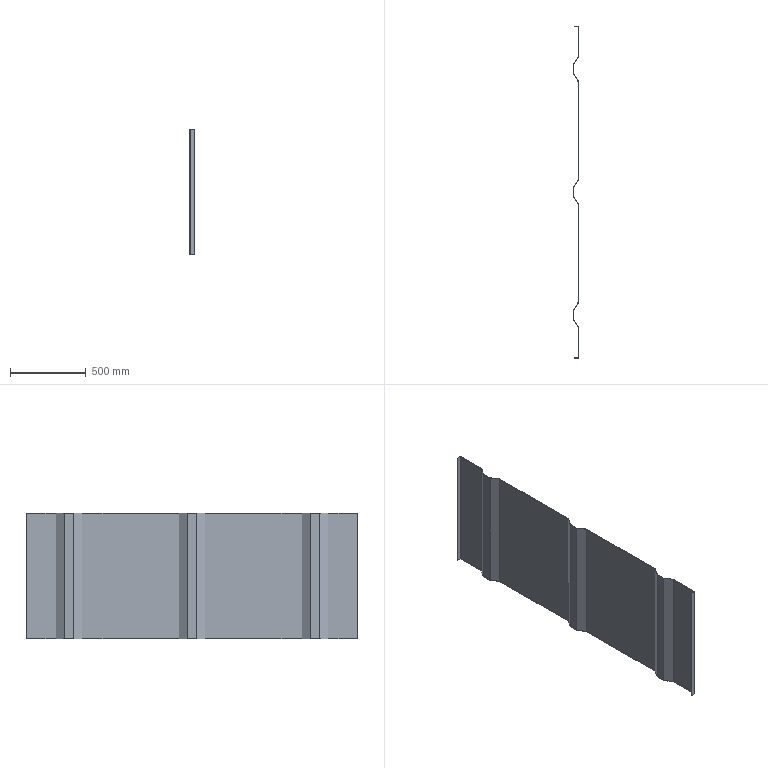Part | SolidWorks | features ExtruThin 1, ICE 1 | 1 solid | 34 faces | box 38 x 2190 x 827 mm | volume 3823055 mm3 | plane 34
STEP:
#1=CARTESIAN_POINT('',(-2.,-1093.,-413.5));
#2=VERTEX_POINT('',#1);
#3=CARTESIAN_POINT('',(-30.,-1093.,-413.5));
#4=VERTEX_POINT('',#3);
#5=CARTESIAN_POINT('',(0.,-1093.,-413.5));
#6=DIRECTION('',(-1.,0.,0.));
#7=VECTOR('',#6,1000.);
#8=LINE('',#5,#7);
#9=EDGE_CURVE('',#2,#4,#8,.T.);
#10=ORIENTED_EDGE('',*,*,#9,.T.);
#11=CARTESIAN_POINT('',(-30.,-1093.,413.5));
#12=VERTEX_POINT('',#11);
#13=CARTESIAN_POINT('',(-30.,-1093.,413.5));
#14=DIRECTION('',(0.,0.,-1.));
#15=VECTOR('',#14,1000.);
#16=LINE('',#13,#15);
#17=EDGE_CURVE('',#12,#4,#16,.T.);
#18=ORIENTED_EDGE('',*,*,#17,.F.);
#19=CARTESIAN_POINT('',(-2.,-1093.,413.5));
#20=VERTEX_POINT('',#19);
#21=CARTESIAN_POINT('',(0.,-1093.,413.5));
#22=DIRECTION('',(-1.,0.,0.));
#23=VECTOR('',#22,1000.);
#24=LINE('',#21,#23);
#25=EDGE_CURVE('',#20,#12,#24,.T.);
#26=ORIENTED_EDGE('',*,*,#25,.F.);
#27=CARTESIAN_POINT('',(-2.,-1093.,413.5));
#28=DIRECTION('',(0.,0.,-1.));
#29=VECTOR('',#28,1000.);
#30=LINE('',#27,#29);
#31=EDGE_CURVE('',#20,#2,#30,.T.);
#32=ORIENTED_EDGE('',*,*,#31,.T.);
#33=EDGE_LOOP('',(#10,#18,#26,#32));
#34=FACE_OUTER_BOUND('',#33,.T.);
#35=CARTESIAN_POINT('',(0.,-1093.,413.5));
#36=DIRECTION('',(0.,-1.,0.));
#37=DIRECTION('',(0.,0.,-1.));
#38=AXIS2_PLACEMENT_3D('',#35,#36,#37);
#39=PLANE('',#38);
#40=ADVANCED_FACE('',(#34),#39,.F.);
#41=CARTESIAN_POINT('',(-30.,-1095.,-413.5));
#42=VERTEX_POINT('',#41);
#43=CARTESIAN_POINT('',(-30.,-1095.,-413.5));
#44=DIRECTION('',(0.,1.,0.));
#45=VECTOR('',#44,1000.);
#46=LINE('',#43,#45);
#47=EDGE_CURVE('',#42,#4,#46,.T.);
#48=ORIENTED_EDGE('',*,*,#47,.F.);
#49=CARTESIAN_POINT('',(-30.,-1095.,413.5));
#50=VERTEX_POINT('',#49);
#51=CARTESIAN_POINT('',(-30.,-1095.,413.5));
#52=DIRECTION('',(0.,0.,-1.));
#53=VECTOR('',#52,1000.);
#54=LINE('',#51,#53);
#55=EDGE_CURVE('',#50,#42,#54,.T.);
#56=ORIENTED_EDGE('',*,*,#55,.F.);
#57=CARTESIAN_POINT('',(-30.,-1095.,413.5));
#58=DIRECTION('',(0.,1.,0.));
#59=VECTOR('',#58,1000.);
#60=LINE('',#57,#59);
#61=EDGE_CURVE('',#50,#12,#60,.T.);
#62=ORIENTED_EDGE('',*,*,#61,.T.);
#63=ORIENTED_EDGE('',*,*,#17,.T.);
#64=EDGE_LOOP('',(#48,#56,#62,#63));
#65=FACE_OUTER_BOUND('',#64,.T.);
#66=CARTESIAN_POINT('',(-30.,-1095.,413.5));
#67=DIRECTION('',(-1.,0.,0.));
#68=DIRECTION('',(0.,0.,1.));
#69=AXIS2_PLACEMENT_3D('',#66,#67,#68);
#70=PLANE('',#69);
#71=ADVANCED_FACE('',(#65),#70,.T.);
#72=CARTESIAN_POINT('',(0.,-1095.,-413.5));
#73=VERTEX_POINT('',#72);
#74=CARTESIAN_POINT('',(0.,-1095.,-413.5));
#75=DIRECTION('',(-1.,0.,0.));
#76=VECTOR('',#75,1000.);
#77=LINE('',#74,#76);
#78=EDGE_CURVE('',#73,#42,#77,.T.);
#79=ORIENTED_EDGE('',*,*,#78,.F.);
#80=CARTESIAN_POINT('',(0.,-1095.,413.5));
#81=VERTEX_POINT('',#80);
#82=CARTESIAN_POINT('',(0.,-1095.,413.5));
#83=DIRECTION('',(0.,0.,-1.));
#84=VECTOR('',#83,1000.);
#85=LINE('',#82,#84);
#86=EDGE_CURVE('',#81,#73,#85,.T.);
#87=ORIENTED_EDGE('',*,*,#86,.F.);
#88=CARTESIAN_POINT('',(0.,-1095.,413.5));
#89=DIRECTION('',(-1.,0.,0.));
#90=VECTOR('',#89,1000.);
#91=LINE('',#88,#90);
#92=EDGE_CURVE('',#81,#50,#91,.T.);
#93=ORIENTED_EDGE('',*,*,#92,.T.);
#94=ORIENTED_EDGE('',*,*,#55,.T.);
#95=EDGE_LOOP('',(#79,#87,#93,#94));
#96=FACE_OUTER_BOUND('',#95,.T.);
#97=CARTESIAN_POINT('',(0.,-1095.,413.5));
#98=DIRECTION('',(0.,-1.,0.));
#99=DIRECTION('',(0.,0.,-1.));
#100=AXIS2_PLACEMENT_3D('',#97,#98,#99);
#101=PLANE('',#100);
#102=ADVANCED_FACE('',(#96),#101,.T.);
#103=CARTESIAN_POINT('',(0.,-895.,-413.5));
#104=VERTEX_POINT('',#103);
#105=CARTESIAN_POINT('',(0.,-895.,-413.5));
#106=DIRECTION('',(0.,-1.,0.));
#107=VECTOR('',#106,1000.);
#108=LINE('',#105,#107);
#109=EDGE_CURVE('',#104,#73,#108,.T.);
#110=ORIENTED_EDGE('',*,*,#109,.F.);
#111=CARTESIAN_POINT('',(0.,-895.,413.5));
#112=VERTEX_POINT('',#111);
#113=CARTESIAN_POINT('',(0.,-895.,413.5));
#114=DIRECTION('',(0.,0.,-1.));
#115=VECTOR('',#114,1000.);
#116=LINE('',#113,#115);
#117=EDGE_CURVE('',#112,#104,#116,.T.);
#118=ORIENTED_EDGE('',*,*,#117,.F.);
#119=CARTESIAN_POINT('',(0.,-895.,413.5));
#120=DIRECTION('',(0.,-1.,0.));
#121=VECTOR('',#120,1000.);
#122=LINE('',#119,#121);
#123=EDGE_CURVE('',#112,#81,#122,.T.);
#124=ORIENTED_EDGE('',*,*,#123,.T.);
#125=ORIENTED_EDGE('',*,*,#86,.T.);
#126=EDGE_LOOP('',(#110,#118,#124,#125));
#127=FACE_OUTER_BOUND('',#126,.T.);
#128=CARTESIAN_POINT('',(0.,-895.,413.5));
#129=DIRECTION('',(1.,0.,0.));
#130=DIRECTION('',(0.,1.,0.));
#131=AXIS2_PLACEMENT_3D('',#128,#129,#130);
#132=PLANE('',#131);
#133=ADVANCED_FACE('',(#127),#132,.T.);
#134=CARTESIAN_POINT('',(-36.,-841.,-413.5));
#135=VERTEX_POINT('',#134);
#136=CARTESIAN_POINT('',(0.,-895.,-413.5));
#137=DIRECTION('',(0.5547,-0.8321,0.));
#138=VECTOR('',#137,1000.);
#139=LINE('',#136,#138);
#140=EDGE_CURVE('',#135,#104,#139,.T.);
#141=ORIENTED_EDGE('',*,*,#140,.F.);
#142=CARTESIAN_POINT('',(-36.,-841.,413.5));
#143=VERTEX_POINT('',#142);
#144=CARTESIAN_POINT('',(-36.,-841.,413.5));
#145=DIRECTION('',(0.,0.,-1.));
#146=VECTOR('',#145,1000.);
#147=LINE('',#144,#146);
#148=EDGE_CURVE('',#143,#135,#147,.T.);
#149=ORIENTED_EDGE('',*,*,#148,.F.);
#150=CARTESIAN_POINT('',(0.,-895.,413.5));
#151=DIRECTION('',(0.5547,-0.8321,0.));
#152=VECTOR('',#151,1000.);
#153=LINE('',#150,#152);
#154=EDGE_CURVE('',#143,#112,#153,.T.);
#155=ORIENTED_EDGE('',*,*,#154,.T.);
#156=ORIENTED_EDGE('',*,*,#117,.T.);
#157=EDGE_LOOP('',(#141,#149,#155,#156));
#158=FACE_OUTER_BOUND('',#157,.T.);
#159=CARTESIAN_POINT('',(0.,-895.,413.5));
#160=DIRECTION('',(0.8321,0.5547,0.));
#161=DIRECTION('',(-0.5547,0.8321,0.));
#162=AXIS2_PLACEMENT_3D('',#159,#160,#161);
#163=PLANE('',#162);
#164=ADVANCED_FACE('',(#158),#163,.T.);
#165=CARTESIAN_POINT('',(-36.,-781.,-413.5));
#166=VERTEX_POINT('',#165);
#167=CARTESIAN_POINT('',(-36.,-841.,-413.5));
#168=DIRECTION('',(0.,-1.,0.));
#169=VECTOR('',#168,1000.);
#170=LINE('',#167,#169);
#171=EDGE_CURVE('',#166,#135,#170,.T.);
#172=ORIENTED_EDGE('',*,*,#171,.F.);
#173=CARTESIAN_POINT('',(-36.,-781.,413.5));
#174=VERTEX_POINT('',#173);
#175=CARTESIAN_POINT('',(-36.,-781.,413.5));
#176=DIRECTION('',(0.,0.,-1.));
#177=VECTOR('',#176,1000.);
#178=LINE('',#175,#177);
#179=EDGE_CURVE('',#174,#166,#178,.T.);
#180=ORIENTED_EDGE('',*,*,#179,.F.);
#181=CARTESIAN_POINT('',(-36.,-841.,413.5));
#182=DIRECTION('',(0.,-1.,0.));
#183=VECTOR('',#182,1000.);
#184=LINE('',#181,#183);
#185=EDGE_CURVE('',#174,#143,#184,.T.);
#186=ORIENTED_EDGE('',*,*,#185,.T.);
#187=ORIENTED_EDGE('',*,*,#148,.T.);
#188=EDGE_LOOP('',(#172,#180,#186,#187));
#189=FACE_OUTER_BOUND('',#188,.T.);
#190=CARTESIAN_POINT('',(-36.,-841.,413.5));
#191=DIRECTION('',(1.,0.,0.));
#192=DIRECTION('',(0.,1.,0.));
#193=AXIS2_PLACEMENT_3D('',#190,#191,#192);
#194=PLANE('',#193);
#195=ADVANCED_FACE('',(#189),#194,.T.);
#196=CARTESIAN_POINT('',(0.,-727.,-413.5));
#197=VERTEX_POINT('',#196);
#198=CARTESIAN_POINT('',(-36.,-781.,-413.5));
#199=DIRECTION('',(-0.5547,-0.8321,0.));
#200=VECTOR('',#199,1000.);
#201=LINE('',#198,#200);
#202=EDGE_CURVE('',#197,#166,#201,.T.);
#203=ORIENTED_EDGE('',*,*,#202,.F.);
#204=CARTESIAN_POINT('',(0.,-727.,413.5));
#205=VERTEX_POINT('',#204);
#206=CARTESIAN_POINT('',(0.,-727.,413.5));
#207=DIRECTION('',(0.,0.,-1.));
#208=VECTOR('',#207,1000.);
#209=LINE('',#206,#208);
#210=EDGE_CURVE('',#205,#197,#209,.T.);
#211=ORIENTED_EDGE('',*,*,#210,.F.);
#212=CARTESIAN_POINT('',(-36.,-781.,413.5));
#213=DIRECTION('',(-0.5547,-0.8321,0.));
#214=VECTOR('',#213,1000.);
#215=LINE('',#212,#214);
#216=EDGE_CURVE('',#205,#174,#215,.T.);
#217=ORIENTED_EDGE('',*,*,#216,.T.);
#218=ORIENTED_EDGE('',*,*,#179,.T.);
#219=EDGE_LOOP('',(#203,#211,#217,#218));
#220=FACE_OUTER_BOUND('',#219,.T.);
#221=CARTESIAN_POINT('',(-36.,-781.,413.5));
#222=DIRECTION('',(0.8321,-0.5547,0.));
#223=DIRECTION('',(0.5547,0.8321,0.));
#224=AXIS2_PLACEMENT_3D('',#221,#222,#223);
#225=PLANE('',#224);
#226=ADVANCED_FACE('',(#220),#225,.T.);
#227=CARTESIAN_POINT('',(0.,-84.,-413.5));
#228=VERTEX_POINT('',#227);
#229=CARTESIAN_POINT('',(0.,-84.,-413.5));
#230=DIRECTION('',(0.,-1.,0.));
#231=VECTOR('',#230,1000.);
#232=LINE('',#229,#231);
#233=EDGE_CURVE('',#228,#197,#232,.T.);
#234=ORIENTED_EDGE('',*,*,#233,.F.);
#235=CARTESIAN_POINT('',(0.,-84.,413.5));
#236=VERTEX_POINT('',#235);
#237=CARTESIAN_POINT('',(0.,-84.,413.5));
#238=DIRECTION('',(0.,0.,-1.));
#239=VECTOR('',#238,1000.);
#240=LINE('',#237,#239);
#241=EDGE_CURVE('',#236,#228,#240,.T.);
#242=ORIENTED_EDGE('',*,*,#241,.F.);
#243=CARTESIAN_POINT('',(0.,-84.,413.5));
#244=DIRECTION('',(0.,-1.,0.));
#245=VECTOR('',#244,1000.);
#246=LINE('',#243,#245);
#247=EDGE_CURVE('',#236,#205,#246,.T.);
#248=ORIENTED_EDGE('',*,*,#247,.T.);
#249=ORIENTED_EDGE('',*,*,#210,.T.);
#250=EDGE_LOOP('',(#234,#242,#248,#249));
#251=FACE_OUTER_BOUND('',#250,.T.);
#252=CARTESIAN_POINT('',(0.,-84.,413.5));
#253=DIRECTION('',(1.,0.,0.));
#254=DIRECTION('',(0.,1.,0.));
#255=AXIS2_PLACEMENT_3D('',#252,#253,#254);
#256=PLANE('',#255);
#257=ADVANCED_FACE('',(#251),#256,.T.);
#258=CARTESIAN_POINT('',(-36.,-30.,-413.5));
#259=VERTEX_POINT('',#258);
#260=CARTESIAN_POINT('',(-36.,-30.,-413.5));
#261=DIRECTION('',(0.5547,-0.8321,0.));
#262=VECTOR('',#261,1000.);
#263=LINE('',#260,#262);
#264=EDGE_CURVE('',#259,#228,#263,.T.);
#265=ORIENTED_EDGE('',*,*,#264,.F.);
#266=CARTESIAN_POINT('',(-36.,-30.,413.5));
#267=VERTEX_POINT('',#266);
#268=CARTESIAN_POINT('',(-36.,-30.,413.5));
#269=DIRECTION('',(0.,0.,-1.));
#270=VECTOR('',#269,1000.);
#271=LINE('',#268,#270);
#272=EDGE_CURVE('',#267,#259,#271,.T.);
#273=ORIENTED_EDGE('',*,*,#272,.F.);
#274=CARTESIAN_POINT('',(-36.,-30.,413.5));
#275=DIRECTION('',(0.5547,-0.8321,0.));
#276=VECTOR('',#275,1000.);
#277=LINE('',#274,#276);
#278=EDGE_CURVE('',#267,#236,#277,.T.);
#279=ORIENTED_EDGE('',*,*,#278,.T.);
#280=ORIENTED_EDGE('',*,*,#241,.T.);
#281=EDGE_LOOP('',(#265,#273,#279,#280));
#282=FACE_OUTER_BOUND('',#281,.T.);
#283=CARTESIAN_POINT('',(-36.,-30.,413.5));
#284=DIRECTION('',(0.8321,0.5547,0.));
#285=DIRECTION('',(-0.5547,0.8321,0.));
#286=AXIS2_PLACEMENT_3D('',#283,#284,#285);
#287=PLANE('',#286);
#288=ADVANCED_FACE('',(#282),#287,.T.);
#289=CARTESIAN_POINT('',(-36.,30.,-413.5));
#290=VERTEX_POINT('',#289);
#291=CARTESIAN_POINT('',(-36.,30.,-413.5));
#292=DIRECTION('',(0.,-1.,0.));
#293=VECTOR('',#292,1000.);
#294=LINE('',#291,#293);
#295=EDGE_CURVE('',#290,#259,#294,.T.);
#296=ORIENTED_EDGE('',*,*,#295,.F.);
#297=CARTESIAN_POINT('',(-36.,30.,413.5));
#298=VERTEX_POINT('',#297);
#299=CARTESIAN_POINT('',(-36.,30.,413.5));
#300=DIRECTION('',(0.,0.,-1.));
#301=VECTOR('',#300,1000.);
#302=LINE('',#299,#301);
#303=EDGE_CURVE('',#298,#290,#302,.T.);
#304=ORIENTED_EDGE('',*,*,#303,.F.);
#305=CARTESIAN_POINT('',(-36.,30.,413.5));
#306=DIRECTION('',(0.,-1.,0.));
#307=VECTOR('',#306,1000.);
#308=LINE('',#305,#307);
#309=EDGE_CURVE('',#298,#267,#308,.T.);
#310=ORIENTED_EDGE('',*,*,#309,.T.);
#311=ORIENTED_EDGE('',*,*,#272,.T.);
#312=EDGE_LOOP('',(#296,#304,#310,#311));
#313=FACE_OUTER_BOUND('',#312,.T.);
#314=CARTESIAN_POINT('',(-36.,30.,413.5));
#315=DIRECTION('',(1.,0.,0.));
#316=DIRECTION('',(0.,1.,0.));
#317=AXIS2_PLACEMENT_3D('',#314,#315,#316);
#318=PLANE('',#317);
#319=ADVANCED_FACE('',(#313),#318,.T.);
#320=CARTESIAN_POINT('',(0.,84.,-413.5));
#321=VERTEX_POINT('',#320);
#322=CARTESIAN_POINT('',(0.,84.,-413.5));
#323=DIRECTION('',(-0.5547,-0.8321,0.));
#324=VECTOR('',#323,1000.);
#325=LINE('',#322,#324);
#326=EDGE_CURVE('',#321,#290,#325,.T.);
#327=ORIENTED_EDGE('',*,*,#326,.F.);
#328=CARTESIAN_POINT('',(0.,84.,413.5));
#329=VERTEX_POINT('',#328);
#330=CARTESIAN_POINT('',(0.,84.,413.5));
#331=DIRECTION('',(0.,0.,-1.));
#332=VECTOR('',#331,1000.);
#333=LINE('',#330,#332);
#334=EDGE_CURVE('',#329,#321,#333,.T.);
#335=ORIENTED_EDGE('',*,*,#334,.F.);
#336=CARTESIAN_POINT('',(0.,84.,413.5));
#337=DIRECTION('',(-0.5547,-0.8321,0.));
#338=VECTOR('',#337,1000.);
#339=LINE('',#336,#338);
#340=EDGE_CURVE('',#329,#298,#339,.T.);
#341=ORIENTED_EDGE('',*,*,#340,.T.);
#342=ORIENTED_EDGE('',*,*,#303,.T.);
#343=EDGE_LOOP('',(#327,#335,#341,#342));
#344=FACE_OUTER_BOUND('',#343,.T.);
#345=CARTESIAN_POINT('',(0.,84.,413.5));
#346=DIRECTION('',(0.8321,-0.5547,0.));
#347=DIRECTION('',(0.5547,0.8321,0.));
#348=AXIS2_PLACEMENT_3D('',#345,#346,#347);
#349=PLANE('',#348);
#350=ADVANCED_FACE('',(#344),#349,.T.);
#351=CARTESIAN_POINT('',(0.,727.,-413.5));
#352=VERTEX_POINT('',#351);
#353=CARTESIAN_POINT('',(0.,727.,-413.5));
#354=DIRECTION('',(0.,-1.,0.));
#355=VECTOR('',#354,1000.);
#356=LINE('',#353,#355);
#357=EDGE_CURVE('',#352,#321,#356,.T.);
#358=ORIENTED_EDGE('',*,*,#357,.F.);
#359=CARTESIAN_POINT('',(0.,727.,413.5));
#360=VERTEX_POINT('',#359);
#361=CARTESIAN_POINT('',(0.,727.,413.5));
#362=DIRECTION('',(0.,0.,-1.));
#363=VECTOR('',#362,1000.);
#364=LINE('',#361,#363);
#365=EDGE_CURVE('',#360,#352,#364,.T.);
#366=ORIENTED_EDGE('',*,*,#365,.F.);
#367=CARTESIAN_POINT('',(0.,727.,413.5));
#368=DIRECTION('',(0.,-1.,0.));
#369=VECTOR('',#368,1000.);
#370=LINE('',#367,#369);
#371=EDGE_CURVE('',#360,#329,#370,.T.);
#372=ORIENTED_EDGE('',*,*,#371,.T.);
#373=ORIENTED_EDGE('',*,*,#334,.T.);
#374=EDGE_LOOP('',(#358,#366,#372,#373));
#375=FACE_OUTER_BOUND('',#374,.T.);
#376=CARTESIAN_POINT('',(0.,727.,413.5));
#377=DIRECTION('',(1.,0.,0.));
#378=DIRECTION('',(0.,1.,0.));
#379=AXIS2_PLACEMENT_3D('',#376,#377,#378);
#380=PLANE('',#379);
#381=ADVANCED_FACE('',(#375),#380,.T.);
#382=CARTESIAN_POINT('',(-36.,781.,-413.5));
#383=VERTEX_POINT('',#382);
#384=CARTESIAN_POINT('',(-36.,781.,-413.5));
#385=DIRECTION('',(0.5547,-0.8321,0.));
#386=VECTOR('',#385,1000.);
#387=LINE('',#384,#386);
#388=EDGE_CURVE('',#383,#352,#387,.T.);
#389=ORIENTED_EDGE('',*,*,#388,.F.);
#390=CARTESIAN_POINT('',(-36.,781.,413.5));
#391=VERTEX_POINT('',#390);
#392=CARTESIAN_POINT('',(-36.,781.,413.5));
#393=DIRECTION('',(0.,0.,-1.));
#394=VECTOR('',#393,1000.);
#395=LINE('',#392,#394);
#396=EDGE_CURVE('',#391,#383,#395,.T.);
#397=ORIENTED_EDGE('',*,*,#396,.F.);
#398=CARTESIAN_POINT('',(-36.,781.,413.5));
#399=DIRECTION('',(0.5547,-0.8321,0.));
#400=VECTOR('',#399,1000.);
#401=LINE('',#398,#400);
#402=EDGE_CURVE('',#391,#360,#401,.T.);
#403=ORIENTED_EDGE('',*,*,#402,.T.);
#404=ORIENTED_EDGE('',*,*,#365,.T.);
#405=EDGE_LOOP('',(#389,#397,#403,#404));
#406=FACE_OUTER_BOUND('',#405,.T.);
#407=CARTESIAN_POINT('',(-36.,781.,413.5));
#408=DIRECTION('',(0.8321,0.5547,0.));
#409=DIRECTION('',(-0.5547,0.8321,0.));
#410=AXIS2_PLACEMENT_3D('',#407,#408,#409);
#411=PLANE('',#410);
#412=ADVANCED_FACE('',(#406),#411,.T.);
#413=CARTESIAN_POINT('',(-36.,841.,-413.5));
#414=VERTEX_POINT('',#413);
#415=CARTESIAN_POINT('',(-36.,841.,-413.5));
#416=DIRECTION('',(0.,-1.,0.));
#417=VECTOR('',#416,1000.);
#418=LINE('',#415,#417);
#419=EDGE_CURVE('',#414,#383,#418,.T.);
#420=ORIENTED_EDGE('',*,*,#419,.F.);
#421=CARTESIAN_POINT('',(-36.,841.,413.5));
#422=VERTEX_POINT('',#421);
#423=CARTESIAN_POINT('',(-36.,841.,413.5));
#424=DIRECTION('',(0.,0.,-1.));
#425=VECTOR('',#424,1000.);
#426=LINE('',#423,#425);
#427=EDGE_CURVE('',#422,#414,#426,.T.);
#428=ORIENTED_EDGE('',*,*,#427,.F.);
#429=CARTESIAN_POINT('',(-36.,841.,413.5));
#430=DIRECTION('',(0.,-1.,0.));
#431=VECTOR('',#430,1000.);
#432=LINE('',#429,#431);
#433=EDGE_CURVE('',#422,#391,#432,.T.);
#434=ORIENTED_EDGE('',*,*,#433,.T.);
#435=ORIENTED_EDGE('',*,*,#396,.T.);
#436=EDGE_LOOP('',(#420,#428,#434,#435));
#437=FACE_OUTER_BOUND('',#436,.T.);
#438=CARTESIAN_POINT('',(-36.,841.,413.5));
#439=DIRECTION('',(1.,0.,0.));
#440=DIRECTION('',(0.,1.,0.));
#441=AXIS2_PLACEMENT_3D('',#438,#439,#440);
#442=PLANE('',#441);
#443=ADVANCED_FACE('',(#437),#442,.T.);
#444=CARTESIAN_POINT('',(0.,895.,-413.5));
#445=VERTEX_POINT('',#444);
#446=CARTESIAN_POINT('',(0.,895.,-413.5));
#447=DIRECTION('',(-0.5547,-0.8321,0.));
#448=VECTOR('',#447,1000.);
#449=LINE('',#446,#448);
#450=EDGE_CURVE('',#445,#414,#449,.T.);
#451=ORIENTED_EDGE('',*,*,#450,.F.);
#452=CARTESIAN_POINT('',(0.,895.,413.5));
#453=VERTEX_POINT('',#452);
#454=CARTESIAN_POINT('',(0.,895.,413.5));
#455=DIRECTION('',(0.,0.,-1.));
#456=VECTOR('',#455,1000.);
#457=LINE('',#454,#456);
#458=EDGE_CURVE('',#453,#445,#457,.T.);
#459=ORIENTED_EDGE('',*,*,#458,.F.);
#460=CARTESIAN_POINT('',(0.,895.,413.5));
#461=DIRECTION('',(-0.5547,-0.8321,0.));
#462=VECTOR('',#461,1000.);
#463=LINE('',#460,#462);
#464=EDGE_CURVE('',#453,#422,#463,.T.);
#465=ORIENTED_EDGE('',*,*,#464,.T.);
#466=ORIENTED_EDGE('',*,*,#427,.T.);
#467=EDGE_LOOP('',(#451,#459,#465,#466));
#468=FACE_OUTER_BOUND('',#467,.T.);
#469=CARTESIAN_POINT('',(0.,895.,413.5));
#470=DIRECTION('',(0.8321,-0.5547,0.));
#471=DIRECTION('',(0.5547,0.8321,0.));
#472=AXIS2_PLACEMENT_3D('',#469,#470,#471);
#473=PLANE('',#472);
#474=ADVANCED_FACE('',(#468),#473,.T.);
#475=CARTESIAN_POINT('',(0.,1095.,-413.5));
#476=VERTEX_POINT('',#475);
#477=CARTESIAN_POINT('',(0.,1095.,-413.5));
#478=DIRECTION('',(0.,-1.,0.));
#479=VECTOR('',#478,1000.);
#480=LINE('',#477,#479);
#481=EDGE_CURVE('',#476,#445,#480,.T.);
#482=ORIENTED_EDGE('',*,*,#481,.F.);
#483=CARTESIAN_POINT('',(0.,1095.,413.5));
#484=VERTEX_POINT('',#483);
#485=CARTESIAN_POINT('',(0.,1095.,413.5));
#486=DIRECTION('',(0.,0.,-1.));
#487=VECTOR('',#486,1000.);
#488=LINE('',#485,#487);
#489=EDGE_CURVE('',#484,#476,#488,.T.);
#490=ORIENTED_EDGE('',*,*,#489,.F.);
#491=CARTESIAN_POINT('',(0.,1095.,413.5));
#492=DIRECTION('',(0.,-1.,0.));
#493=VECTOR('',#492,1000.);
#494=LINE('',#491,#493);
#495=EDGE_CURVE('',#484,#453,#494,.T.);
#496=ORIENTED_EDGE('',*,*,#495,.T.);
#497=ORIENTED_EDGE('',*,*,#458,.T.);
#498=EDGE_LOOP('',(#482,#490,#496,#497));
#499=FACE_OUTER_BOUND('',#498,.T.);
#500=CARTESIAN_POINT('',(0.,1095.,413.5));
#501=DIRECTION('',(1.,0.,0.));
#502=DIRECTION('',(0.,1.,0.));
#503=AXIS2_PLACEMENT_3D('',#500,#501,#502);
#504=PLANE('',#503);
#505=ADVANCED_FACE('',(#499),#504,.T.);
#506=CARTESIAN_POINT('',(-30.,1095.,-413.5));
#507=VERTEX_POINT('',#506);
#508=CARTESIAN_POINT('',(0.,1095.,-413.5));
#509=DIRECTION('',(1.,0.,0.));
#510=VECTOR('',#509,1000.);
#511=LINE('',#508,#510);
#512=EDGE_CURVE('',#507,#476,#511,.T.);
#513=ORIENTED_EDGE('',*,*,#512,.F.);
#514=CARTESIAN_POINT('',(-30.,1095.,413.5));
#515=VERTEX_POINT('',#514);
#516=CARTESIAN_POINT('',(-30.,1095.,413.5));
#517=DIRECTION('',(0.,0.,-1.));
#518=VECTOR('',#517,1000.);
#519=LINE('',#516,#518);
#520=EDGE_CURVE('',#515,#507,#519,.T.);
#521=ORIENTED_EDGE('',*,*,#520,.F.);
#522=CARTESIAN_POINT('',(0.,1095.,413.5));
#523=DIRECTION('',(1.,0.,0.));
#524=VECTOR('',#523,1000.);
#525=LINE('',#522,#524);
#526=EDGE_CURVE('',#515,#484,#525,.T.);
#527=ORIENTED_EDGE('',*,*,#526,.T.);
#528=ORIENTED_EDGE('',*,*,#489,.T.);
#529=EDGE_LOOP('',(#513,#521,#527,#528));
#530=FACE_OUTER_BOUND('',#529,.T.);
#531=CARTESIAN_POINT('',(0.,1095.,413.5));
#532=DIRECTION('',(0.,1.,0.));
#533=DIRECTION('',(0.,0.,1.));
#534=AXIS2_PLACEMENT_3D('',#531,#532,#533);
#535=PLANE('',#534);
#536=ADVANCED_FACE('',(#530),#535,.T.);
#537=CARTESIAN_POINT('',(-30.,1093.,-413.5));
#538=VERTEX_POINT('',#537);
#539=CARTESIAN_POINT('',(-30.,1093.,-413.5));
#540=DIRECTION('',(0.,1.,0.));
#541=VECTOR('',#540,1000.);
#542=LINE('',#539,#541);
#543=EDGE_CURVE('',#538,#507,#542,.T.);
#544=ORIENTED_EDGE('',*,*,#543,.F.);
#545=CARTESIAN_POINT('',(-30.,1093.,413.5));
#546=VERTEX_POINT('',#545);
#547=CARTESIAN_POINT('',(-30.,1093.,413.5));
#548=DIRECTION('',(0.,0.,-1.));
#549=VECTOR('',#548,1000.);
#550=LINE('',#547,#549);
#551=EDGE_CURVE('',#546,#538,#550,.T.);
#552=ORIENTED_EDGE('',*,*,#551,.F.);
#553=CARTESIAN_POINT('',(-30.,1093.,413.5));
#554=DIRECTION('',(0.,1.,0.));
#555=VECTOR('',#554,1000.);
#556=LINE('',#553,#555);
#557=EDGE_CURVE('',#546,#515,#556,.T.);
#558=ORIENTED_EDGE('',*,*,#557,.T.);
#559=ORIENTED_EDGE('',*,*,#520,.T.);
#560=EDGE_LOOP('',(#544,#552,#558,#559));
#561=FACE_OUTER_BOUND('',#560,.T.);
#562=CARTESIAN_POINT('',(-30.,1093.,413.5));
#563=DIRECTION('',(-1.,0.,0.));
#564=DIRECTION('',(0.,0.,1.));
#565=AXIS2_PLACEMENT_3D('',#562,#563,#564);
#566=PLANE('',#565);
#567=ADVANCED_FACE('',(#561),#566,.T.);
#568=CARTESIAN_POINT('',(-2.,1093.,-413.5));
#569=VERTEX_POINT('',#568);
#570=CARTESIAN_POINT('',(0.,1093.,-413.5));
#571=DIRECTION('',(1.,0.,0.));
#572=VECTOR('',#571,1000.);
#573=LINE('',#570,#572);
#574=EDGE_CURVE('',#538,#569,#573,.T.);
#575=ORIENTED_EDGE('',*,*,#574,.T.);
#576=CARTESIAN_POINT('',(-2.,1093.,413.5));
#577=VERTEX_POINT('',#576);
#578=CARTESIAN_POINT('',(-2.,1093.,413.5));
#579=DIRECTION('',(0.,0.,-1.));
#580=VECTOR('',#579,1000.);
#581=LINE('',#578,#580);
#582=EDGE_CURVE('',#577,#569,#581,.T.);
#583=ORIENTED_EDGE('',*,*,#582,.F.);
#584=CARTESIAN_POINT('',(0.,1093.,413.5));
#585=DIRECTION('',(1.,0.,0.));
#586=VECTOR('',#585,1000.);
#587=LINE('',#584,#586);
#588=EDGE_CURVE('',#546,#577,#587,.T.);
#589=ORIENTED_EDGE('',*,*,#588,.F.);
#590=ORIENTED_EDGE('',*,*,#551,.T.);
#591=EDGE_LOOP('',(#575,#583,#589,#590));
#592=FACE_OUTER_BOUND('',#591,.T.);
#593=CARTESIAN_POINT('',(0.,1093.,413.5));
#594=DIRECTION('',(0.,1.,0.));
#595=DIRECTION('',(0.,0.,1.));
#596=AXIS2_PLACEMENT_3D('',#593,#594,#595);
#597=PLANE('',#596);
#598=ADVANCED_FACE('',(#592),#597,.F.);
#599=CARTESIAN_POINT('',(-2.,895.606,-413.5));
#600=VERTEX_POINT('',#599);
#601=CARTESIAN_POINT('',(-2.,1095.,-413.5));
#602=DIRECTION('',(0.,-1.,0.));
#603=VECTOR('',#602,1000.);
#604=LINE('',#601,#603);
#605=EDGE_CURVE('',#569,#600,#604,.T.);
#606=ORIENTED_EDGE('',*,*,#605,.T.);
#607=CARTESIAN_POINT('',(-2.,895.606,413.5));
#608=VERTEX_POINT('',#607);
#609=CARTESIAN_POINT('',(-2.,895.606,413.5));
#610=DIRECTION('',(0.,0.,-1.));
#611=VECTOR('',#610,1000.);
#612=LINE('',#609,#611);
#613=EDGE_CURVE('',#608,#600,#612,.T.);
#614=ORIENTED_EDGE('',*,*,#613,.F.);
#615=CARTESIAN_POINT('',(-2.,1095.,413.5));
#616=DIRECTION('',(0.,-1.,0.));
#617=VECTOR('',#616,1000.);
#618=LINE('',#615,#617);
#619=EDGE_CURVE('',#577,#608,#618,.T.);
#620=ORIENTED_EDGE('',*,*,#619,.F.);
#621=ORIENTED_EDGE('',*,*,#582,.T.);
#622=EDGE_LOOP('',(#606,#614,#620,#621));
#623=FACE_OUTER_BOUND('',#622,.T.);
#624=CARTESIAN_POINT('',(-2.,1095.,413.5));
#625=DIRECTION('',(1.,0.,0.));
#626=DIRECTION('',(0.,1.,0.));
#627=AXIS2_PLACEMENT_3D('',#624,#625,#626);
#628=PLANE('',#627);
#629=ADVANCED_FACE('',(#623),#628,.F.);
#630=CARTESIAN_POINT('',(-38.,841.606,-413.5));
#631=VERTEX_POINT('',#630);
#632=CARTESIAN_POINT('',(-1.664,896.109,-413.5));
#633=DIRECTION('',(-0.5547,-0.8321,0.));
#634=VECTOR('',#633,1000.);
#635=LINE('',#632,#634);
#636=EDGE_CURVE('',#600,#631,#635,.T.);
#637=ORIENTED_EDGE('',*,*,#636,.T.);
#638=CARTESIAN_POINT('',(-38.,841.606,413.5));
#639=VERTEX_POINT('',#638);
#640=CARTESIAN_POINT('',(-38.,841.606,413.5));
#641=DIRECTION('',(0.,0.,-1.));
#642=VECTOR('',#641,1000.);
#643=LINE('',#640,#642);
#644=EDGE_CURVE('',#639,#631,#643,.T.);
#645=ORIENTED_EDGE('',*,*,#644,.F.);
#646=CARTESIAN_POINT('',(-1.664,896.109,413.5));
#647=DIRECTION('',(-0.5547,-0.8321,0.));
#648=VECTOR('',#647,1000.);
#649=LINE('',#646,#648);
#650=EDGE_CURVE('',#608,#639,#649,.T.);
#651=ORIENTED_EDGE('',*,*,#650,.F.);
#652=ORIENTED_EDGE('',*,*,#613,.T.);
#653=EDGE_LOOP('',(#637,#645,#651,#652));
#654=FACE_OUTER_BOUND('',#653,.T.);
#655=CARTESIAN_POINT('',(-1.664,896.109,413.5));
#656=DIRECTION('',(0.8321,-0.5547,0.));
#657=DIRECTION('',(0.5547,0.8321,0.));
#658=AXIS2_PLACEMENT_3D('',#655,#656,#657);
#659=PLANE('',#658);
#660=ADVANCED_FACE('',(#654),#659,.F.);
#661=CARTESIAN_POINT('',(-38.,780.394,-413.5));
#662=VERTEX_POINT('',#661);
#663=CARTESIAN_POINT('',(-38.,841.,-413.5));
#664=DIRECTION('',(0.,-1.,0.));
#665=VECTOR('',#664,1000.);
#666=LINE('',#663,#665);
#667=EDGE_CURVE('',#631,#662,#666,.T.);
#668=ORIENTED_EDGE('',*,*,#667,.T.);
#669=CARTESIAN_POINT('',(-38.,780.394,413.5));
#670=VERTEX_POINT('',#669);
#671=CARTESIAN_POINT('',(-38.,780.394,413.5));
#672=DIRECTION('',(0.,0.,-1.));
#673=VECTOR('',#672,1000.);
#674=LINE('',#671,#673);
#675=EDGE_CURVE('',#670,#662,#674,.T.);
#676=ORIENTED_EDGE('',*,*,#675,.F.);
#677=CARTESIAN_POINT('',(-38.,841.,413.5));
#678=DIRECTION('',(0.,-1.,0.));
#679=VECTOR('',#678,1000.);
#680=LINE('',#677,#679);
#681=EDGE_CURVE('',#639,#670,#680,.T.);
#682=ORIENTED_EDGE('',*,*,#681,.F.);
#683=ORIENTED_EDGE('',*,*,#644,.T.);
#684=EDGE_LOOP('',(#668,#676,#682,#683));
#685=FACE_OUTER_BOUND('',#684,.T.);
#686=CARTESIAN_POINT('',(-38.,841.,413.5));
#687=DIRECTION('',(1.,0.,0.));
#688=DIRECTION('',(0.,1.,0.));
#689=AXIS2_PLACEMENT_3D('',#686,#687,#688);
#690=PLANE('',#689);
#691=ADVANCED_FACE('',(#685),#690,.F.);
#692=CARTESIAN_POINT('',(-2.,726.394,-413.5));
#693=VERTEX_POINT('',#692);
#694=CARTESIAN_POINT('',(-37.664,779.891,-413.5));
#695=DIRECTION('',(0.5547,-0.8321,0.));
#696=VECTOR('',#695,1000.);
#697=LINE('',#694,#696);
#698=EDGE_CURVE('',#662,#693,#697,.T.);
#699=ORIENTED_EDGE('',*,*,#698,.T.);
#700=CARTESIAN_POINT('',(-2.,726.394,413.5));
#701=VERTEX_POINT('',#700);
#702=CARTESIAN_POINT('',(-2.,726.394,413.5));
#703=DIRECTION('',(0.,0.,-1.));
#704=VECTOR('',#703,1000.);
#705=LINE('',#702,#704);
#706=EDGE_CURVE('',#701,#693,#705,.T.);
#707=ORIENTED_EDGE('',*,*,#706,.F.);
#708=CARTESIAN_POINT('',(-37.664,779.891,413.5));
#709=DIRECTION('',(0.5547,-0.8321,0.));
#710=VECTOR('',#709,1000.);
#711=LINE('',#708,#710);
#712=EDGE_CURVE('',#670,#701,#711,.T.);
#713=ORIENTED_EDGE('',*,*,#712,.F.);
#714=ORIENTED_EDGE('',*,*,#675,.T.);
#715=EDGE_LOOP('',(#699,#707,#713,#714));
#716=FACE_OUTER_BOUND('',#715,.T.);
#717=CARTESIAN_POINT('',(-37.664,779.891,413.5));
#718=DIRECTION('',(0.8321,0.5547,0.));
#719=DIRECTION('',(-0.5547,0.8321,0.));
#720=AXIS2_PLACEMENT_3D('',#717,#718,#719);
#721=PLANE('',#720);
#722=ADVANCED_FACE('',(#716),#721,.F.);
#723=CARTESIAN_POINT('',(-2.,84.606,-413.5));
#724=VERTEX_POINT('',#723);
#725=CARTESIAN_POINT('',(-2.,727.,-413.5));
#726=DIRECTION('',(0.,-1.,0.));
#727=VECTOR('',#726,1000.);
#728=LINE('',#725,#727);
#729=EDGE_CURVE('',#693,#724,#728,.T.);
#730=ORIENTED_EDGE('',*,*,#729,.T.);
#731=CARTESIAN_POINT('',(-2.,84.606,413.5));
#732=VERTEX_POINT('',#731);
#733=CARTESIAN_POINT('',(-2.,84.606,413.5));
#734=DIRECTION('',(0.,0.,-1.));
#735=VECTOR('',#734,1000.);
#736=LINE('',#733,#735);
#737=EDGE_CURVE('',#732,#724,#736,.T.);
#738=ORIENTED_EDGE('',*,*,#737,.F.);
#739=CARTESIAN_POINT('',(-2.,727.,413.5));
#740=DIRECTION('',(0.,-1.,0.));
#741=VECTOR('',#740,1000.);
#742=LINE('',#739,#741);
#743=EDGE_CURVE('',#701,#732,#742,.T.);
#744=ORIENTED_EDGE('',*,*,#743,.F.);
#745=ORIENTED_EDGE('',*,*,#706,.T.);
#746=EDGE_LOOP('',(#730,#738,#744,#745));
#747=FACE_OUTER_BOUND('',#746,.T.);
#748=CARTESIAN_POINT('',(-2.,727.,413.5));
#749=DIRECTION('',(1.,0.,0.));
#750=DIRECTION('',(0.,1.,0.));
#751=AXIS2_PLACEMENT_3D('',#748,#749,#750);
#752=PLANE('',#751);
#753=ADVANCED_FACE('',(#747),#752,.F.);
#754=CARTESIAN_POINT('',(-38.,30.606,-413.5));
#755=VERTEX_POINT('',#754);
#756=CARTESIAN_POINT('',(-1.664,85.109,-413.5));
#757=DIRECTION('',(-0.5547,-0.8321,0.));
#758=VECTOR('',#757,1000.);
#759=LINE('',#756,#758);
#760=EDGE_CURVE('',#724,#755,#759,.T.);
#761=ORIENTED_EDGE('',*,*,#760,.T.);
#762=CARTESIAN_POINT('',(-38.,30.606,413.5));
#763=VERTEX_POINT('',#762);
#764=CARTESIAN_POINT('',(-38.,30.606,413.5));
#765=DIRECTION('',(0.,0.,-1.));
#766=VECTOR('',#765,1000.);
#767=LINE('',#764,#766);
#768=EDGE_CURVE('',#763,#755,#767,.T.);
#769=ORIENTED_EDGE('',*,*,#768,.F.);
#770=CARTESIAN_POINT('',(-1.664,85.109,413.5));
#771=DIRECTION('',(-0.5547,-0.8321,0.));
#772=VECTOR('',#771,1000.);
#773=LINE('',#770,#772);
#774=EDGE_CURVE('',#732,#763,#773,.T.);
#775=ORIENTED_EDGE('',*,*,#774,.F.);
#776=ORIENTED_EDGE('',*,*,#737,.T.);
#777=EDGE_LOOP('',(#761,#769,#775,#776));
#778=FACE_OUTER_BOUND('',#777,.T.);
#779=CARTESIAN_POINT('',(-1.664,85.109,413.5));
#780=DIRECTION('',(0.8321,-0.5547,0.));
#781=DIRECTION('',(0.5547,0.8321,0.));
#782=AXIS2_PLACEMENT_3D('',#779,#780,#781);
#783=PLANE('',#782);
#784=ADVANCED_FACE('',(#778),#783,.F.);
#785=CARTESIAN_POINT('',(-38.,-30.606,-413.5));
#786=VERTEX_POINT('',#785);
#787=CARTESIAN_POINT('',(-38.,30.,-413.5));
#788=DIRECTION('',(0.,-1.,0.));
#789=VECTOR('',#788,1000.);
#790=LINE('',#787,#789);
#791=EDGE_CURVE('',#755,#786,#790,.T.);
#792=ORIENTED_EDGE('',*,*,#791,.T.);
#793=CARTESIAN_POINT('',(-38.,-30.606,413.5));
#794=VERTEX_POINT('',#793);
#795=CARTESIAN_POINT('',(-38.,-30.606,413.5));
#796=DIRECTION('',(0.,0.,-1.));
#797=VECTOR('',#796,1000.);
#798=LINE('',#795,#797);
#799=EDGE_CURVE('',#794,#786,#798,.T.);
#800=ORIENTED_EDGE('',*,*,#799,.F.);
#801=CARTESIAN_POINT('',(-38.,30.,413.5));
#802=DIRECTION('',(0.,-1.,0.));
#803=VECTOR('',#802,1000.);
#804=LINE('',#801,#803);
#805=EDGE_CURVE('',#763,#794,#804,.T.);
#806=ORIENTED_EDGE('',*,*,#805,.F.);
#807=ORIENTED_EDGE('',*,*,#768,.T.);
#808=EDGE_LOOP('',(#792,#800,#806,#807));
#809=FACE_OUTER_BOUND('',#808,.T.);
#810=CARTESIAN_POINT('',(-38.,30.,413.5));
#811=DIRECTION('',(1.,0.,0.));
#812=DIRECTION('',(0.,1.,0.));
#813=AXIS2_PLACEMENT_3D('',#810,#811,#812);
#814=PLANE('',#813);
#815=ADVANCED_FACE('',(#809),#814,.F.);
#816=CARTESIAN_POINT('',(-2.,-84.606,-413.5));
#817=VERTEX_POINT('',#816);
#818=CARTESIAN_POINT('',(-37.664,-31.109,-413.5));
#819=DIRECTION('',(0.5547,-0.8321,0.));
#820=VECTOR('',#819,1000.);
#821=LINE('',#818,#820);
#822=EDGE_CURVE('',#786,#817,#821,.T.);
#823=ORIENTED_EDGE('',*,*,#822,.T.);
#824=CARTESIAN_POINT('',(-2.,-84.606,413.5));
#825=VERTEX_POINT('',#824);
#826=CARTESIAN_POINT('',(-2.,-84.606,413.5));
#827=DIRECTION('',(0.,0.,-1.));
#828=VECTOR('',#827,1000.);
#829=LINE('',#826,#828);
#830=EDGE_CURVE('',#825,#817,#829,.T.);
#831=ORIENTED_EDGE('',*,*,#830,.F.);
#832=CARTESIAN_POINT('',(-37.664,-31.109,413.5));
#833=DIRECTION('',(0.5547,-0.8321,0.));
#834=VECTOR('',#833,1000.);
#835=LINE('',#832,#834);
#836=EDGE_CURVE('',#794,#825,#835,.T.);
#837=ORIENTED_EDGE('',*,*,#836,.F.);
#838=ORIENTED_EDGE('',*,*,#799,.T.);
#839=EDGE_LOOP('',(#823,#831,#837,#838));
#840=FACE_OUTER_BOUND('',#839,.T.);
#841=CARTESIAN_POINT('',(-37.664,-31.109,413.5));
#842=DIRECTION('',(0.8321,0.5547,0.));
#843=DIRECTION('',(-0.5547,0.8321,0.));
#844=AXIS2_PLACEMENT_3D('',#841,#842,#843);
#845=PLANE('',#844);
#846=ADVANCED_FACE('',(#840),#845,.F.);
#847=CARTESIAN_POINT('',(-2.,-726.394,-413.5));
#848=VERTEX_POINT('',#847);
#849=CARTESIAN_POINT('',(-2.,-84.,-413.5));
#850=DIRECTION('',(0.,-1.,0.));
#851=VECTOR('',#850,1000.);
#852=LINE('',#849,#851);
#853=EDGE_CURVE('',#817,#848,#852,.T.);
#854=ORIENTED_EDGE('',*,*,#853,.T.);
#855=CARTESIAN_POINT('',(-2.,-726.394,413.5));
#856=VERTEX_POINT('',#855);
#857=CARTESIAN_POINT('',(-2.,-726.394,413.5));
#858=DIRECTION('',(0.,0.,-1.));
#859=VECTOR('',#858,1000.);
#860=LINE('',#857,#859);
#861=EDGE_CURVE('',#856,#848,#860,.T.);
#862=ORIENTED_EDGE('',*,*,#861,.F.);
#863=CARTESIAN_POINT('',(-2.,-84.,413.5));
#864=DIRECTION('',(0.,-1.,0.));
#865=VECTOR('',#864,1000.);
#866=LINE('',#863,#865);
#867=EDGE_CURVE('',#825,#856,#866,.T.);
#868=ORIENTED_EDGE('',*,*,#867,.F.);
#869=ORIENTED_EDGE('',*,*,#830,.T.);
#870=EDGE_LOOP('',(#854,#862,#868,#869));
#871=FACE_OUTER_BOUND('',#870,.T.);
#872=CARTESIAN_POINT('',(-2.,-84.,413.5));
#873=DIRECTION('',(1.,0.,0.));
#874=DIRECTION('',(0.,1.,0.));
#875=AXIS2_PLACEMENT_3D('',#872,#873,#874);
#876=PLANE('',#875);
#877=ADVANCED_FACE('',(#871),#876,.F.);
#878=CARTESIAN_POINT('',(-38.,-780.394,-413.5));
#879=VERTEX_POINT('',#878);
#880=CARTESIAN_POINT('',(-37.664,-779.891,-413.5));
#881=DIRECTION('',(-0.5547,-0.8321,0.));
#882=VECTOR('',#881,1000.);
#883=LINE('',#880,#882);
#884=EDGE_CURVE('',#848,#879,#883,.T.);
#885=ORIENTED_EDGE('',*,*,#884,.T.);
#886=CARTESIAN_POINT('',(-38.,-780.394,413.5));
#887=VERTEX_POINT('',#886);
#888=CARTESIAN_POINT('',(-38.,-780.394,413.5));
#889=DIRECTION('',(0.,0.,-1.));
#890=VECTOR('',#889,1000.);
#891=LINE('',#888,#890);
#892=EDGE_CURVE('',#887,#879,#891,.T.);
#893=ORIENTED_EDGE('',*,*,#892,.F.);
#894=CARTESIAN_POINT('',(-37.664,-779.891,413.5));
#895=DIRECTION('',(-0.5547,-0.8321,0.));
#896=VECTOR('',#895,1000.);
#897=LINE('',#894,#896);
#898=EDGE_CURVE('',#856,#887,#897,.T.);
#899=ORIENTED_EDGE('',*,*,#898,.F.);
#900=ORIENTED_EDGE('',*,*,#861,.T.);
#901=EDGE_LOOP('',(#885,#893,#899,#900));
#902=FACE_OUTER_BOUND('',#901,.T.);
#903=CARTESIAN_POINT('',(-37.664,-779.891,413.5));
#904=DIRECTION('',(0.8321,-0.5547,0.));
#905=DIRECTION('',(0.5547,0.8321,0.));
#906=AXIS2_PLACEMENT_3D('',#903,#904,#905);
#907=PLANE('',#906);
#908=ADVANCED_FACE('',(#902),#907,.F.);
#909=CARTESIAN_POINT('',(-38.,-841.606,-413.5));
#910=VERTEX_POINT('',#909);
#911=CARTESIAN_POINT('',(-38.,-841.,-413.5));
#912=DIRECTION('',(0.,-1.,0.));
#913=VECTOR('',#912,1000.);
#914=LINE('',#911,#913);
#915=EDGE_CURVE('',#879,#910,#914,.T.);
#916=ORIENTED_EDGE('',*,*,#915,.T.);
#917=CARTESIAN_POINT('',(-38.,-841.606,413.5));
#918=VERTEX_POINT('',#917);
#919=CARTESIAN_POINT('',(-38.,-841.606,413.5));
#920=DIRECTION('',(0.,0.,-1.));
#921=VECTOR('',#920,1000.);
#922=LINE('',#919,#921);
#923=EDGE_CURVE('',#918,#910,#922,.T.);
#924=ORIENTED_EDGE('',*,*,#923,.F.);
#925=CARTESIAN_POINT('',(-38.,-841.,413.5));
#926=DIRECTION('',(0.,-1.,0.));
#927=VECTOR('',#926,1000.);
#928=LINE('',#925,#927);
#929=EDGE_CURVE('',#887,#918,#928,.T.);
#930=ORIENTED_EDGE('',*,*,#929,.F.);
#931=ORIENTED_EDGE('',*,*,#892,.T.);
#932=EDGE_LOOP('',(#916,#924,#930,#931));
#933=FACE_OUTER_BOUND('',#932,.T.);
#934=CARTESIAN_POINT('',(-38.,-841.,413.5));
#935=DIRECTION('',(1.,0.,0.));
#936=DIRECTION('',(0.,1.,0.));
#937=AXIS2_PLACEMENT_3D('',#934,#935,#936);
#938=PLANE('',#937);
#939=ADVANCED_FACE('',(#933),#938,.F.);
#940=CARTESIAN_POINT('',(-2.,-895.606,-413.5));
#941=VERTEX_POINT('',#940);
#942=CARTESIAN_POINT('',(-1.664,-896.109,-413.5));
#943=DIRECTION('',(0.5547,-0.8321,0.));
#944=VECTOR('',#943,1000.);
#945=LINE('',#942,#944);
#946=EDGE_CURVE('',#910,#941,#945,.T.);
#947=ORIENTED_EDGE('',*,*,#946,.T.);
#948=CARTESIAN_POINT('',(-2.,-895.606,413.5));
#949=VERTEX_POINT('',#948);
#950=CARTESIAN_POINT('',(-2.,-895.606,413.5));
#951=DIRECTION('',(0.,0.,-1.));
#952=VECTOR('',#951,1000.);
#953=LINE('',#950,#952);
#954=EDGE_CURVE('',#949,#941,#953,.T.);
#955=ORIENTED_EDGE('',*,*,#954,.F.);
#956=CARTESIAN_POINT('',(-1.664,-896.109,413.5));
#957=DIRECTION('',(0.5547,-0.8321,0.));
#958=VECTOR('',#957,1000.);
#959=LINE('',#956,#958);
#960=EDGE_CURVE('',#918,#949,#959,.T.);
#961=ORIENTED_EDGE('',*,*,#960,.F.);
#962=ORIENTED_EDGE('',*,*,#923,.T.);
#963=EDGE_LOOP('',(#947,#955,#961,#962));
#964=FACE_OUTER_BOUND('',#963,.T.);
#965=CARTESIAN_POINT('',(-1.664,-896.109,413.5));
#966=DIRECTION('',(0.8321,0.5547,0.));
#967=DIRECTION('',(-0.5547,0.8321,0.));
#968=AXIS2_PLACEMENT_3D('',#965,#966,#967);
#969=PLANE('',#968);
#970=ADVANCED_FACE('',(#964),#969,.F.);
#971=CARTESIAN_POINT('',(-2.,-895.,-413.5));
#972=DIRECTION('',(0.,-1.,0.));
#973=VECTOR('',#972,1000.);
#974=LINE('',#971,#973);
#975=EDGE_CURVE('',#941,#2,#974,.T.);
#976=ORIENTED_EDGE('',*,*,#975,.T.);
#977=ORIENTED_EDGE('',*,*,#31,.F.);
#978=CARTESIAN_POINT('',(-2.,-895.,413.5));
#979=DIRECTION('',(0.,-1.,0.));
#980=VECTOR('',#979,1000.);
#981=LINE('',#978,#980);
#982=EDGE_CURVE('',#949,#20,#981,.T.);
#983=ORIENTED_EDGE('',*,*,#982,.F.);
#984=ORIENTED_EDGE('',*,*,#954,.T.);
#985=EDGE_LOOP('',(#976,#977,#983,#984));
#986=FACE_OUTER_BOUND('',#985,.T.);
#987=CARTESIAN_POINT('',(-2.,-895.,413.5));
#988=DIRECTION('',(1.,0.,0.));
#989=DIRECTION('',(0.,1.,0.));
#990=AXIS2_PLACEMENT_3D('',#987,#988,#989);
#991=PLANE('',#990);
#992=ADVANCED_FACE('',(#986),#991,.F.);
#993=ORIENTED_EDGE('',*,*,#25,.T.);
#994=ORIENTED_EDGE('',*,*,#61,.F.);
#995=ORIENTED_EDGE('',*,*,#92,.F.);
#996=ORIENTED_EDGE('',*,*,#123,.F.);
#997=ORIENTED_EDGE('',*,*,#154,.F.);
#998=ORIENTED_EDGE('',*,*,#185,.F.);
#999=ORIENTED_EDGE('',*,*,#216,.F.);
#1000=ORIENTED_EDGE('',*,*,#247,.F.);
#1001=ORIENTED_EDGE('',*,*,#278,.F.);
#1002=ORIENTED_EDGE('',*,*,#309,.F.);
#1003=ORIENTED_EDGE('',*,*,#340,.F.);
#1004=ORIENTED_EDGE('',*,*,#371,.F.);
#1005=ORIENTED_EDGE('',*,*,#402,.F.);
#1006=ORIENTED_EDGE('',*,*,#433,.F.);
#1007=ORIENTED_EDGE('',*,*,#464,.F.);
#1008=ORIENTED_EDGE('',*,*,#495,.F.);
#1009=ORIENTED_EDGE('',*,*,#526,.F.);
#1010=ORIENTED_EDGE('',*,*,#557,.F.);
#1011=ORIENTED_EDGE('',*,*,#588,.T.);
#1012=ORIENTED_EDGE('',*,*,#619,.T.);
#1013=ORIENTED_EDGE('',*,*,#650,.T.);
#1014=ORIENTED_EDGE('',*,*,#681,.T.);
#1015=ORIENTED_EDGE('',*,*,#712,.T.);
#1016=ORIENTED_EDGE('',*,*,#743,.T.);
#1017=ORIENTED_EDGE('',*,*,#774,.T.);
#1018=ORIENTED_EDGE('',*,*,#805,.T.);
#1019=ORIENTED_EDGE('',*,*,#836,.T.);
#1020=ORIENTED_EDGE('',*,*,#867,.T.);
#1021=ORIENTED_EDGE('',*,*,#898,.T.);
#1022=ORIENTED_EDGE('',*,*,#929,.T.);
#1023=ORIENTED_EDGE('',*,*,#960,.T.);
#1024=ORIENTED_EDGE('',*,*,#982,.T.);
#1025=EDGE_LOOP('',(#993,#994,#995,#996,#997,#998,#999,#1000,#1001,#1002,#1003,#1004,#1005,#1006,#1007,#1008,#1009,#1010,#1011,#1012,#1013,#1014,#1015,#1016,#1017,#1018,#1019,#1020,#1021,#1022,#1023,#1024));
#1026=FACE_OUTER_BOUND('',#1025,.T.);
#1027=CARTESIAN_POINT('',(0.,0.,413.5));
#1028=DIRECTION('',(0.,0.,1.));
#1029=DIRECTION('',(1.,0.,0.));
#1030=AXIS2_PLACEMENT_3D('',#1027,#1028,#1029);
#1031=PLANE('',#1030);
#1032=ADVANCED_FACE('',(#1026),#1031,.T.);
#1033=ORIENTED_EDGE('',*,*,#9,.F.);
#1034=ORIENTED_EDGE('',*,*,#975,.F.);
#1035=ORIENTED_EDGE('',*,*,#946,.F.);
#1036=ORIENTED_EDGE('',*,*,#915,.F.);
#1037=ORIENTED_EDGE('',*,*,#884,.F.);
#1038=ORIENTED_EDGE('',*,*,#853,.F.);
#1039=ORIENTED_EDGE('',*,*,#822,.F.);
#1040=ORIENTED_EDGE('',*,*,#791,.F.);
#1041=ORIENTED_EDGE('',*,*,#760,.F.);
#1042=ORIENTED_EDGE('',*,*,#729,.F.);
#1043=ORIENTED_EDGE('',*,*,#698,.F.);
#1044=ORIENTED_EDGE('',*,*,#667,.F.);
#1045=ORIENTED_EDGE('',*,*,#636,.F.);
#1046=ORIENTED_EDGE('',*,*,#605,.F.);
#1047=ORIENTED_EDGE('',*,*,#574,.F.);
#1048=ORIENTED_EDGE('',*,*,#543,.T.);
#1049=ORIENTED_EDGE('',*,*,#512,.T.);
#1050=ORIENTED_EDGE('',*,*,#481,.T.);
#1051=ORIENTED_EDGE('',*,*,#450,.T.);
#1052=ORIENTED_EDGE('',*,*,#419,.T.);
#1053=ORIENTED_EDGE('',*,*,#388,.T.);
#1054=ORIENTED_EDGE('',*,*,#357,.T.);
#1055=ORIENTED_EDGE('',*,*,#326,.T.);
#1056=ORIENTED_EDGE('',*,*,#295,.T.);
#1057=ORIENTED_EDGE('',*,*,#264,.T.);
#1058=ORIENTED_EDGE('',*,*,#233,.T.);
#1059=ORIENTED_EDGE('',*,*,#202,.T.);
#1060=ORIENTED_EDGE('',*,*,#171,.T.);
#1061=ORIENTED_EDGE('',*,*,#140,.T.);
#1062=ORIENTED_EDGE('',*,*,#109,.T.);
#1063=ORIENTED_EDGE('',*,*,#78,.T.);
#1064=ORIENTED_EDGE('',*,*,#47,.T.);
#1065=EDGE_LOOP('',(#1033,#1034,#1035,#1036,#1037,#1038,#1039,#1040,#1041,#1042,#1043,#1044,#1045,#1046,#1047,#1048,#1049,#1050,#1051,#1052,#1053,#1054,#1055,#1056,#1057,#1058,#1059,#1060,#1061,#1062,#1063,#1064));
#1066=FACE_OUTER_BOUND('',#1065,.T.);
#1067=CARTESIAN_POINT('',(0.,0.,-413.5));
#1068=DIRECTION('',(0.,0.,1.));
#1069=DIRECTION('',(1.,0.,0.));
#1070=AXIS2_PLACEMENT_3D('',#1067,#1068,#1069);
#1071=PLANE('',#1070);
#1072=ADVANCED_FACE('',(#1066),#1071,.F.);
#1073=CLOSED_SHELL('',(#40,#71,#102,#133,#164,#195,#226,#257,#288,#319,#350,#381,#412,#443,#474,#505,#536,#567,#598,#629,#660,#691,#722,#753,#784,#815,#846,#877,#908,#939,#970,#992,#1032,#1072));
#1074=MANIFOLD_SOLID_BREP('',#1073);
#1075=CARTESIAN_POINT('',(0.,0.,0.));
#1076=DIRECTION('',(0.,0.,1.));
#1077=DIRECTION('',(1.,0.,0.));
#1078=AXIS2_PLACEMENT_3D('',#1075,#1076,#1077);
#1079=(LENGTH_UNIT()NAMED_UNIT(*)SI_UNIT(.MILLI.,.METRE.));
#1080=UNCERTAINTY_MEASURE_WITH_UNIT(LENGTH_MEASURE(0.00001),#1079,'','');
#1081=(NAMED_UNIT(*)PLANE_ANGLE_UNIT()SI_UNIT($,.RADIAN.));
#1082=(NAMED_UNIT(*)SI_UNIT($,.STERADIAN.)SOLID_ANGLE_UNIT());
#1083=(GEOMETRIC_REPRESENTATION_CONTEXT(3)GLOBAL_UNCERTAINTY_ASSIGNED_CONTEXT((#1080))GLOBAL_UNIT_ASSIGNED_CONTEXT((#1079,#1081,#1082))REPRESENTATION_CONTEXT('',''));
#1084=ADVANCED_BREP_SHAPE_REPRESENTATION('',(#1074,#1078),#1083);